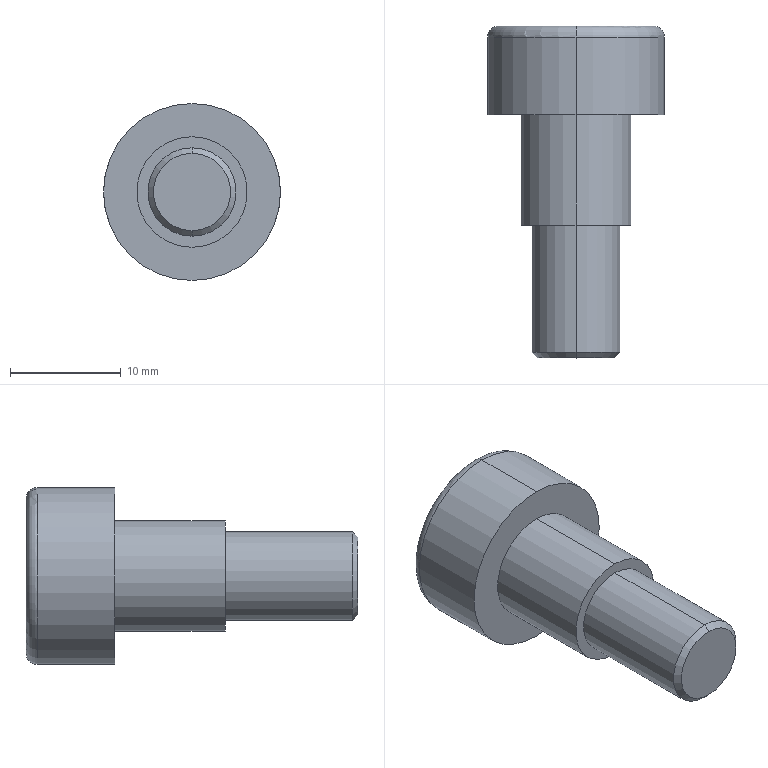Part | STEP file | External thread shoulder bolt MSB10-10 | 1 solid | 21 faces | box 16 x 30 x 16 mm | volume 2915 mm3 | plane 11 | cylinder 6 | torus 2 | cone 2 | commonest cylinder face diameters 8 x2 10 x2 16 x2
STEP:
#1=CARTESIAN_POINT('',(0.,0.,0.));
#2=DIRECTION('',(0.,0.,1.));
#3=DIRECTION('',(1.,0.,0.));
#4=AXIS2_PLACEMENT_3D('',#1,#2,#3);
#5=CARTESIAN_POINT('',(0.,29.,-8.));
#6=VERTEX_POINT('',#5);
#7=CARTESIAN_POINT('',(0.,29.,8.));
#8=VERTEX_POINT('',#7);
#9=CARTESIAN_POINT('',(0.,29.,0.));
#10=DIRECTION('',(0.,-1.,0.));
#11=DIRECTION('',(0.,0.,1.));
#12=AXIS2_PLACEMENT_3D('',#9,#10,#11);
#13=CIRCLE('',#12,8.);
#14=CARTESIAN_POINT('',(0.,29.,0.));
#15=DIRECTION('',(0.,1.,0.));
#16=DIRECTION('',(0.,0.,1.));
#17=AXIS2_PLACEMENT_3D('',#14,#15,#16);
#18=TOROIDAL_SURFACE('',#17,7.,1.);
#19=CARTESIAN_POINT('',(6.283,0.));
#20=DIRECTION('',(-1.,0.));
#21=VECTOR('',#20,1.);
#22=LINE('',#19,#21);
#23=(GEOMETRIC_REPRESENTATION_CONTEXT(2)PARAMETRIC_REPRESENTATION_CONTEXT()REPRESENTATION_CONTEXT('',''));
#24=DEFINITIONAL_REPRESENTATION('',(#22),#23);
#25=PCURVE('',#18,#24);
#26=CARTESIAN_POINT('',(0.,0.,0.));
#27=DIRECTION('',(0.,-1.,0.));
#28=DIRECTION('',(0.,0.,-1.));
#29=AXIS2_PLACEMENT_3D('',#26,#27,#28);
#30=CYLINDRICAL_SURFACE('',#29,8.);
#31=CARTESIAN_POINT('',(-3.142,-29.));
#32=DIRECTION('',(1.,0.));
#33=VECTOR('',#32,1.);
#34=LINE('',#31,#33);
#35=(GEOMETRIC_REPRESENTATION_CONTEXT(2)PARAMETRIC_REPRESENTATION_CONTEXT()REPRESENTATION_CONTEXT('',''));
#36=DEFINITIONAL_REPRESENTATION('',(#34),#35);
#37=PCURVE('',#30,#36);
#38=SURFACE_CURVE('',#13,(#25,#37),.PCURVE_S1.);
#39=EDGE_CURVE('',#6,#8,#38,.T.);
#40=ORIENTED_EDGE('',*,*,#39,.F.);
#41=CARTESIAN_POINT('',(0.,30.,-7.));
#42=VERTEX_POINT('',#41);
#43=CARTESIAN_POINT('',(0.,29.,-7.));
#44=DIRECTION('',(1.,0.,0.));
#45=DIRECTION('',(0.,0.,-1.));
#46=AXIS2_PLACEMENT_3D('',#43,#44,#45);
#47=CIRCLE('',#46,1.);
#48=CARTESIAN_POINT('',(3.142,0.));
#49=DIRECTION('',(0.,1.));
#50=VECTOR('',#49,1.);
#51=LINE('',#48,#50);
#52=(GEOMETRIC_REPRESENTATION_CONTEXT(2)PARAMETRIC_REPRESENTATION_CONTEXT()REPRESENTATION_CONTEXT('',''));
#53=DEFINITIONAL_REPRESENTATION('',(#51),#52);
#54=PCURVE('',#18,#53);
#55=CARTESIAN_POINT('',(0.,29.,0.));
#56=DIRECTION('',(0.,1.,0.));
#57=DIRECTION('',(0.,0.,1.));
#58=AXIS2_PLACEMENT_3D('',#55,#56,#57);
#59=TOROIDAL_SURFACE('',#58,7.,1.);
#60=CARTESIAN_POINT('',(3.142,0.));
#61=DIRECTION('',(0.,1.));
#62=VECTOR('',#61,1.);
#63=LINE('',#60,#62);
#64=(GEOMETRIC_REPRESENTATION_CONTEXT(2)PARAMETRIC_REPRESENTATION_CONTEXT()REPRESENTATION_CONTEXT('',''));
#65=DEFINITIONAL_REPRESENTATION('',(#63),#64);
#66=PCURVE('',#59,#65);
#67=SURFACE_CURVE('',#47,(#54,#66),.PCURVE_S1.);
#68=EDGE_CURVE('',#6,#42,#67,.T.);
#69=ORIENTED_EDGE('',*,*,#68,.T.);
#70=CARTESIAN_POINT('',(0.,30.,7.));
#71=VERTEX_POINT('',#70);
#72=CARTESIAN_POINT('',(0.,30.,0.));
#73=DIRECTION('',(0.,1.,0.));
#74=DIRECTION('',(0.,0.,1.));
#75=AXIS2_PLACEMENT_3D('',#72,#73,#74);
#76=CIRCLE('',#75,7.);
#77=CARTESIAN_POINT('',(0.,1.571));
#78=DIRECTION('',(1.,0.));
#79=VECTOR('',#78,1.);
#80=LINE('',#77,#79);
#81=(GEOMETRIC_REPRESENTATION_CONTEXT(2)PARAMETRIC_REPRESENTATION_CONTEXT()REPRESENTATION_CONTEXT('',''));
#82=DEFINITIONAL_REPRESENTATION('',(#80),#81);
#83=PCURVE('',#18,#82);
#84=CARTESIAN_POINT('',(0.,30.,0.));
#85=DIRECTION('',(0.,1.,0.));
#86=DIRECTION('',(0.,0.,1.));
#87=AXIS2_PLACEMENT_3D('',#84,#85,#86);
#88=PLANE('',#87);
#89=CARTESIAN_POINT('',(0.,0.));
#90=DIRECTION('',(1.,0.));
#91=AXIS2_PLACEMENT_2D('',#89,#90);
#92=CIRCLE('',#91,7.);
#93=(GEOMETRIC_REPRESENTATION_CONTEXT(2)PARAMETRIC_REPRESENTATION_CONTEXT()REPRESENTATION_CONTEXT('',''));
#94=DEFINITIONAL_REPRESENTATION('',(#92),#93);
#95=PCURVE('',#88,#94);
#96=SURFACE_CURVE('',#76,(#83,#95),.PCURVE_S1.);
#97=EDGE_CURVE('',#71,#42,#96,.T.);
#98=ORIENTED_EDGE('',*,*,#97,.F.);
#99=CARTESIAN_POINT('',(0.,29.,7.));
#100=DIRECTION('',(-1.,0.,0.));
#101=DIRECTION('',(0.,0.,1.));
#102=AXIS2_PLACEMENT_3D('',#99,#100,#101);
#103=CIRCLE('',#102,1.);
#104=CARTESIAN_POINT('',(0.,0.));
#105=DIRECTION('',(0.,1.));
#106=VECTOR('',#105,1.);
#107=LINE('',#104,#106);
#108=(GEOMETRIC_REPRESENTATION_CONTEXT(2)PARAMETRIC_REPRESENTATION_CONTEXT()REPRESENTATION_CONTEXT('',''));
#109=DEFINITIONAL_REPRESENTATION('',(#107),#108);
#110=PCURVE('',#18,#109);
#111=CARTESIAN_POINT('',(6.283,0.));
#112=DIRECTION('',(0.,1.));
#113=VECTOR('',#112,1.);
#114=LINE('',#111,#113);
#115=(GEOMETRIC_REPRESENTATION_CONTEXT(2)PARAMETRIC_REPRESENTATION_CONTEXT()REPRESENTATION_CONTEXT('',''));
#116=DEFINITIONAL_REPRESENTATION('',(#114),#115);
#117=PCURVE('',#59,#116);
#118=SURFACE_CURVE('',#103,(#110,#117),.PCURVE_S1.);
#119=EDGE_CURVE('',#8,#71,#118,.T.);
#120=ORIENTED_EDGE('',*,*,#119,.F.);
#121=EDGE_LOOP('',(#40,#69,#98,#120));
#122=FACE_BOUND('',#121,.T.);
#123=ADVANCED_FACE('',(#122),#18,.T.);
#124=CARTESIAN_POINT('',(0.,0.,-3.5));
#125=VERTEX_POINT('',#124);
#126=CARTESIAN_POINT('',(0.,0.,3.5));
#127=VERTEX_POINT('',#126);
#128=CARTESIAN_POINT('',(0.,0.,0.));
#129=DIRECTION('',(0.,-1.,0.));
#130=DIRECTION('',(0.,0.,-1.));
#131=AXIS2_PLACEMENT_3D('',#128,#129,#130);
#132=CIRCLE('',#131,3.5);
#133=CARTESIAN_POINT('',(0.,0.,0.));
#134=DIRECTION('',(0.,1.,0.));
#135=DIRECTION('',(0.,0.,1.));
#136=AXIS2_PLACEMENT_3D('',#133,#134,#135);
#137=CONICAL_SURFACE('',#136,3.5,0.7854);
#138=CARTESIAN_POINT('',(3.142,0.));
#139=DIRECTION('',(-1.,0.));
#140=VECTOR('',#139,1.);
#141=LINE('',#138,#140);
#142=(GEOMETRIC_REPRESENTATION_CONTEXT(2)PARAMETRIC_REPRESENTATION_CONTEXT()REPRESENTATION_CONTEXT('',''));
#143=DEFINITIONAL_REPRESENTATION('',(#141),#142);
#144=PCURVE('',#137,#143);
#145=CARTESIAN_POINT('',(4.,0.,0.));
#146=DIRECTION('',(0.,-1.,0.));
#147=DIRECTION('',(0.,0.,-1.));
#148=AXIS2_PLACEMENT_3D('',#145,#146,#147);
#149=PLANE('',#148);
#150=CARTESIAN_POINT('',(0.,-4.));
#151=DIRECTION('',(1.,0.));
#152=AXIS2_PLACEMENT_2D('',#150,#151);
#153=CIRCLE('',#152,3.5);
#154=(GEOMETRIC_REPRESENTATION_CONTEXT(2)PARAMETRIC_REPRESENTATION_CONTEXT()REPRESENTATION_CONTEXT('',''));
#155=DEFINITIONAL_REPRESENTATION('',(#153),#154);
#156=PCURVE('',#149,#155);
#157=SURFACE_CURVE('',#132,(#144,#156),.PCURVE_S1.);
#158=EDGE_CURVE('',#125,#127,#157,.T.);
#159=ORIENTED_EDGE('',*,*,#158,.F.);
#160=CARTESIAN_POINT('',(0.,0.5,-4.));
#161=VERTEX_POINT('',#160);
#162=CARTESIAN_POINT('',(0.,0.,-3.5));
#163=DIRECTION('',(0.,0.7071,-0.7071));
#164=VECTOR('',#163,1.);
#165=LINE('',#162,#164);
#166=CARTESIAN_POINT('',(3.142,0.));
#167=DIRECTION('',(0.,1.));
#168=VECTOR('',#167,1.);
#169=LINE('',#166,#168);
#170=(GEOMETRIC_REPRESENTATION_CONTEXT(2)PARAMETRIC_REPRESENTATION_CONTEXT()REPRESENTATION_CONTEXT('',''));
#171=DEFINITIONAL_REPRESENTATION('',(#169),#170);
#172=PCURVE('',#137,#171);
#173=CARTESIAN_POINT('',(0.,0.,0.));
#174=DIRECTION('',(0.,1.,0.));
#175=DIRECTION('',(0.,0.,1.));
#176=AXIS2_PLACEMENT_3D('',#173,#174,#175);
#177=CONICAL_SURFACE('',#176,3.5,0.7854);
#178=CARTESIAN_POINT('',(3.142,0.));
#179=DIRECTION('',(0.,1.));
#180=VECTOR('',#179,1.);
#181=LINE('',#178,#180);
#182=(GEOMETRIC_REPRESENTATION_CONTEXT(2)PARAMETRIC_REPRESENTATION_CONTEXT()REPRESENTATION_CONTEXT('',''));
#183=DEFINITIONAL_REPRESENTATION('',(#181),#182);
#184=PCURVE('',#177,#183);
#185=SURFACE_CURVE('',#165,(#172,#184),.PCURVE_S1.);
#186=EDGE_CURVE('',#125,#161,#185,.T.);
#187=ORIENTED_EDGE('',*,*,#186,.T.);
#188=CARTESIAN_POINT('',(0.,0.5,4.));
#189=VERTEX_POINT('',#188);
#190=CARTESIAN_POINT('',(0.,0.5,0.));
#191=DIRECTION('',(0.,1.,0.));
#192=DIRECTION('',(0.,0.,-1.));
#193=AXIS2_PLACEMENT_3D('',#190,#191,#192);
#194=CIRCLE('',#193,4.);
#195=CARTESIAN_POINT('',(-3.142,0.5));
#196=DIRECTION('',(1.,0.));
#197=VECTOR('',#196,1.);
#198=LINE('',#195,#197);
#199=(GEOMETRIC_REPRESENTATION_CONTEXT(2)PARAMETRIC_REPRESENTATION_CONTEXT()REPRESENTATION_CONTEXT('',''));
#200=DEFINITIONAL_REPRESENTATION('',(#198),#199);
#201=PCURVE('',#137,#200);
#202=CARTESIAN_POINT('',(0.,0.,0.));
#203=DIRECTION('',(0.,-1.,0.));
#204=DIRECTION('',(0.,0.,-1.));
#205=AXIS2_PLACEMENT_3D('',#202,#203,#204);
#206=CYLINDRICAL_SURFACE('',#205,4.);
#207=CARTESIAN_POINT('',(6.283,-0.5));
#208=DIRECTION('',(-1.,0.));
#209=VECTOR('',#208,1.);
#210=LINE('',#207,#209);
#211=(GEOMETRIC_REPRESENTATION_CONTEXT(2)PARAMETRIC_REPRESENTATION_CONTEXT()REPRESENTATION_CONTEXT('',''));
#212=DEFINITIONAL_REPRESENTATION('',(#210),#211);
#213=PCURVE('',#206,#212);
#214=SURFACE_CURVE('',#194,(#201,#213),.PCURVE_S1.);
#215=EDGE_CURVE('',#189,#161,#214,.T.);
#216=ORIENTED_EDGE('',*,*,#215,.F.);
#217=CARTESIAN_POINT('',(0.,0.,3.5));
#218=DIRECTION('',(0.,0.7071,0.7071));
#219=VECTOR('',#218,1.);
#220=LINE('',#217,#219);
#221=CARTESIAN_POINT('',(0.,0.));
#222=DIRECTION('',(0.,1.));
#223=VECTOR('',#222,1.);
#224=LINE('',#221,#223);
#225=(GEOMETRIC_REPRESENTATION_CONTEXT(2)PARAMETRIC_REPRESENTATION_CONTEXT()REPRESENTATION_CONTEXT('',''));
#226=DEFINITIONAL_REPRESENTATION('',(#224),#225);
#227=PCURVE('',#137,#226);
#228=CARTESIAN_POINT('',(6.283,0.));
#229=DIRECTION('',(0.,1.));
#230=VECTOR('',#229,1.);
#231=LINE('',#228,#230);
#232=(GEOMETRIC_REPRESENTATION_CONTEXT(2)PARAMETRIC_REPRESENTATION_CONTEXT()REPRESENTATION_CONTEXT('',''));
#233=DEFINITIONAL_REPRESENTATION('',(#231),#232);
#234=PCURVE('',#177,#233);
#235=SURFACE_CURVE('',#220,(#227,#234),.PCURVE_S1.);
#236=EDGE_CURVE('',#127,#189,#235,.T.);
#237=ORIENTED_EDGE('',*,*,#236,.F.);
#238=EDGE_LOOP('',(#159,#187,#216,#237));
#239=FACE_BOUND('',#238,.T.);
#240=ADVANCED_FACE('',(#239),#137,.T.);
#241=CARTESIAN_POINT('',(0.,12.,-4.));
#242=VERTEX_POINT('',#241);
#243=CARTESIAN_POINT('',(0.,12.,4.));
#244=VERTEX_POINT('',#243);
#245=CARTESIAN_POINT('',(0.,12.,0.));
#246=DIRECTION('',(0.,-1.,0.));
#247=DIRECTION('',(0.,0.,-1.));
#248=AXIS2_PLACEMENT_3D('',#245,#246,#247);
#249=CIRCLE('',#248,4.);
#250=CARTESIAN_POINT('',(0.,-12.));
#251=DIRECTION('',(1.,0.));
#252=VECTOR('',#251,1.);
#253=LINE('',#250,#252);
#254=(GEOMETRIC_REPRESENTATION_CONTEXT(2)PARAMETRIC_REPRESENTATION_CONTEXT()REPRESENTATION_CONTEXT('',''));
#255=DEFINITIONAL_REPRESENTATION('',(#253),#254);
#256=PCURVE('',#206,#255);
#257=CARTESIAN_POINT('',(5.,12.,0.));
#258=DIRECTION('',(0.,-1.,0.));
#259=DIRECTION('',(0.,0.,-1.));
#260=AXIS2_PLACEMENT_3D('',#257,#258,#259);
#261=PLANE('',#260);
#262=CARTESIAN_POINT('',(0.,-5.));
#263=DIRECTION('',(1.,0.));
#264=AXIS2_PLACEMENT_2D('',#262,#263);
#265=CIRCLE('',#264,4.);
#266=(GEOMETRIC_REPRESENTATION_CONTEXT(2)PARAMETRIC_REPRESENTATION_CONTEXT()REPRESENTATION_CONTEXT('',''));
#267=DEFINITIONAL_REPRESENTATION('',(#265),#266);
#268=PCURVE('',#261,#267);
#269=SURFACE_CURVE('',#249,(#256,#268),.PCURVE_S1.);
#270=EDGE_CURVE('',#242,#244,#269,.T.);
#271=ORIENTED_EDGE('',*,*,#270,.T.);
#272=CARTESIAN_POINT('',(0.,0.,4.));
#273=DIRECTION('',(0.,-1.,0.));
#274=VECTOR('',#273,1.);
#275=LINE('',#272,#274);
#276=CARTESIAN_POINT('',(3.142,0.));
#277=DIRECTION('',(0.,1.));
#278=VECTOR('',#277,1.);
#279=LINE('',#276,#278);
#280=(GEOMETRIC_REPRESENTATION_CONTEXT(2)PARAMETRIC_REPRESENTATION_CONTEXT()REPRESENTATION_CONTEXT('',''));
#281=DEFINITIONAL_REPRESENTATION('',(#279),#280);
#282=PCURVE('',#206,#281);
#283=CARTESIAN_POINT('',(0.,0.,0.));
#284=DIRECTION('',(0.,-1.,0.));
#285=DIRECTION('',(0.,0.,-1.));
#286=AXIS2_PLACEMENT_3D('',#283,#284,#285);
#287=CYLINDRICAL_SURFACE('',#286,4.);
#288=CARTESIAN_POINT('',(3.142,0.));
#289=DIRECTION('',(0.,1.));
#290=VECTOR('',#289,1.);
#291=LINE('',#288,#290);
#292=(GEOMETRIC_REPRESENTATION_CONTEXT(2)PARAMETRIC_REPRESENTATION_CONTEXT()REPRESENTATION_CONTEXT('',''));
#293=DEFINITIONAL_REPRESENTATION('',(#291),#292);
#294=PCURVE('',#287,#293);
#295=SURFACE_CURVE('',#275,(#282,#294),.PCURVE_S1.);
#296=EDGE_CURVE('',#244,#189,#295,.T.);
#297=ORIENTED_EDGE('',*,*,#296,.T.);
#298=ORIENTED_EDGE('',*,*,#215,.T.);
#299=CARTESIAN_POINT('',(0.,0.,-4.));
#300=DIRECTION('',(0.,-1.,0.));
#301=VECTOR('',#300,1.);
#302=LINE('',#299,#301);
#303=CARTESIAN_POINT('',(0.,0.));
#304=DIRECTION('',(0.,1.));
#305=VECTOR('',#304,1.);
#306=LINE('',#303,#305);
#307=(GEOMETRIC_REPRESENTATION_CONTEXT(2)PARAMETRIC_REPRESENTATION_CONTEXT()REPRESENTATION_CONTEXT('',''));
#308=DEFINITIONAL_REPRESENTATION('',(#306),#307);
#309=PCURVE('',#206,#308);
#310=CARTESIAN_POINT('',(6.283,0.));
#311=DIRECTION('',(0.,1.));
#312=VECTOR('',#311,1.);
#313=LINE('',#310,#312);
#314=(GEOMETRIC_REPRESENTATION_CONTEXT(2)PARAMETRIC_REPRESENTATION_CONTEXT()REPRESENTATION_CONTEXT('',''));
#315=DEFINITIONAL_REPRESENTATION('',(#313),#314);
#316=PCURVE('',#287,#315);
#317=SURFACE_CURVE('',#302,(#309,#316),.PCURVE_S1.);
#318=EDGE_CURVE('',#242,#161,#317,.T.);
#319=ORIENTED_EDGE('',*,*,#318,.F.);
#320=EDGE_LOOP('',(#271,#297,#298,#319));
#321=FACE_BOUND('',#320,.T.);
#322=ADVANCED_FACE('',(#321),#206,.T.);
#323=CARTESIAN_POINT('',(0.,22.,-5.));
#324=VERTEX_POINT('',#323);
#325=CARTESIAN_POINT('',(0.,22.,5.));
#326=VERTEX_POINT('',#325);
#327=CARTESIAN_POINT('',(0.,22.,0.));
#328=DIRECTION('',(0.,-1.,0.));
#329=DIRECTION('',(0.,0.,-1.));
#330=AXIS2_PLACEMENT_3D('',#327,#328,#329);
#331=CIRCLE('',#330,5.);
#332=CARTESIAN_POINT('',(0.,0.,0.));
#333=DIRECTION('',(0.,-1.,0.));
#334=DIRECTION('',(0.,0.,-1.));
#335=AXIS2_PLACEMENT_3D('',#332,#333,#334);
#336=CYLINDRICAL_SURFACE('',#335,5.);
#337=CARTESIAN_POINT('',(0.,-22.));
#338=DIRECTION('',(1.,0.));
#339=VECTOR('',#338,1.);
#340=LINE('',#337,#339);
#341=(GEOMETRIC_REPRESENTATION_CONTEXT(2)PARAMETRIC_REPRESENTATION_CONTEXT()REPRESENTATION_CONTEXT('',''));
#342=DEFINITIONAL_REPRESENTATION('',(#340),#341);
#343=PCURVE('',#336,#342);
#344=CARTESIAN_POINT('',(8.,22.,0.));
#345=DIRECTION('',(0.,-1.,0.));
#346=DIRECTION('',(0.,0.,-1.));
#347=AXIS2_PLACEMENT_3D('',#344,#345,#346);
#348=PLANE('',#347);
#349=CARTESIAN_POINT('',(0.,-8.));
#350=DIRECTION('',(1.,0.));
#351=AXIS2_PLACEMENT_2D('',#349,#350);
#352=CIRCLE('',#351,5.);
#353=(GEOMETRIC_REPRESENTATION_CONTEXT(2)PARAMETRIC_REPRESENTATION_CONTEXT()REPRESENTATION_CONTEXT('',''));
#354=DEFINITIONAL_REPRESENTATION('',(#352),#353);
#355=PCURVE('',#348,#354);
#356=SURFACE_CURVE('',#331,(#343,#355),.PCURVE_S1.);
#357=EDGE_CURVE('',#324,#326,#356,.T.);
#358=ORIENTED_EDGE('',*,*,#357,.T.);
#359=CARTESIAN_POINT('',(0.,12.,5.));
#360=VERTEX_POINT('',#359);
#361=CARTESIAN_POINT('',(0.,0.,5.));
#362=DIRECTION('',(0.,-1.,0.));
#363=VECTOR('',#362,1.);
#364=LINE('',#361,#363);
#365=CARTESIAN_POINT('',(3.142,0.));
#366=DIRECTION('',(0.,1.));
#367=VECTOR('',#366,1.);
#368=LINE('',#365,#367);
#369=(GEOMETRIC_REPRESENTATION_CONTEXT(2)PARAMETRIC_REPRESENTATION_CONTEXT()REPRESENTATION_CONTEXT('',''));
#370=DEFINITIONAL_REPRESENTATION('',(#368),#369);
#371=PCURVE('',#336,#370);
#372=CARTESIAN_POINT('',(0.,0.,0.));
#373=DIRECTION('',(0.,-1.,0.));
#374=DIRECTION('',(0.,0.,-1.));
#375=AXIS2_PLACEMENT_3D('',#372,#373,#374);
#376=CYLINDRICAL_SURFACE('',#375,5.);
#377=CARTESIAN_POINT('',(3.142,0.));
#378=DIRECTION('',(0.,1.));
#379=VECTOR('',#378,1.);
#380=LINE('',#377,#379);
#381=(GEOMETRIC_REPRESENTATION_CONTEXT(2)PARAMETRIC_REPRESENTATION_CONTEXT()REPRESENTATION_CONTEXT('',''));
#382=DEFINITIONAL_REPRESENTATION('',(#380),#381);
#383=PCURVE('',#376,#382);
#384=SURFACE_CURVE('',#364,(#371,#383),.PCURVE_S1.);
#385=EDGE_CURVE('',#326,#360,#384,.T.);
#386=ORIENTED_EDGE('',*,*,#385,.T.);
#387=CARTESIAN_POINT('',(0.,12.,-5.));
#388=VERTEX_POINT('',#387);
#389=CARTESIAN_POINT('',(0.,12.,0.));
#390=DIRECTION('',(0.,-1.,0.));
#391=DIRECTION('',(0.,0.,-1.));
#392=AXIS2_PLACEMENT_3D('',#389,#390,#391);
#393=CIRCLE('',#392,5.);
#394=CARTESIAN_POINT('',(0.,-12.));
#395=DIRECTION('',(1.,0.));
#396=VECTOR('',#395,1.);
#397=LINE('',#394,#396);
#398=(GEOMETRIC_REPRESENTATION_CONTEXT(2)PARAMETRIC_REPRESENTATION_CONTEXT()REPRESENTATION_CONTEXT('',''));
#399=DEFINITIONAL_REPRESENTATION('',(#397),#398);
#400=PCURVE('',#336,#399);
#401=CARTESIAN_POINT('',(0.,-5.));
#402=DIRECTION('',(1.,0.));
#403=AXIS2_PLACEMENT_2D('',#401,#402);
#404=CIRCLE('',#403,5.);
#405=(GEOMETRIC_REPRESENTATION_CONTEXT(2)PARAMETRIC_REPRESENTATION_CONTEXT()REPRESENTATION_CONTEXT('',''));
#406=DEFINITIONAL_REPRESENTATION('',(#404),#405);
#407=PCURVE('',#261,#406);
#408=SURFACE_CURVE('',#393,(#400,#407),.PCURVE_S1.);
#409=EDGE_CURVE('',#388,#360,#408,.T.);
#410=ORIENTED_EDGE('',*,*,#409,.F.);
#411=CARTESIAN_POINT('',(0.,0.,-5.));
#412=DIRECTION('',(0.,-1.,0.));
#413=VECTOR('',#412,1.);
#414=LINE('',#411,#413);
#415=CARTESIAN_POINT('',(0.,0.));
#416=DIRECTION('',(0.,1.));
#417=VECTOR('',#416,1.);
#418=LINE('',#415,#417);
#419=(GEOMETRIC_REPRESENTATION_CONTEXT(2)PARAMETRIC_REPRESENTATION_CONTEXT()REPRESENTATION_CONTEXT('',''));
#420=DEFINITIONAL_REPRESENTATION('',(#418),#419);
#421=PCURVE('',#336,#420);
#422=CARTESIAN_POINT('',(6.283,0.));
#423=DIRECTION('',(0.,1.));
#424=VECTOR('',#423,1.);
#425=LINE('',#422,#424);
#426=(GEOMETRIC_REPRESENTATION_CONTEXT(2)PARAMETRIC_REPRESENTATION_CONTEXT()REPRESENTATION_CONTEXT('',''));
#427=DEFINITIONAL_REPRESENTATION('',(#425),#426);
#428=PCURVE('',#376,#427);
#429=SURFACE_CURVE('',#414,(#421,#428),.PCURVE_S1.);
#430=EDGE_CURVE('',#324,#388,#429,.T.);
#431=ORIENTED_EDGE('',*,*,#430,.F.);
#432=EDGE_LOOP('',(#358,#386,#410,#431));
#433=FACE_BOUND('',#432,.T.);
#434=ADVANCED_FACE('',(#433),#336,.T.);
#435=ORIENTED_EDGE('',*,*,#39,.T.);
#436=CARTESIAN_POINT('',(0.,22.,8.));
#437=VERTEX_POINT('',#436);
#438=CARTESIAN_POINT('',(0.,0.,8.));
#439=DIRECTION('',(0.,-1.,0.));
#440=VECTOR('',#439,1.);
#441=LINE('',#438,#440);
#442=CARTESIAN_POINT('',(3.142,0.));
#443=DIRECTION('',(0.,1.));
#444=VECTOR('',#443,1.);
#445=LINE('',#442,#444);
#446=(GEOMETRIC_REPRESENTATION_CONTEXT(2)PARAMETRIC_REPRESENTATION_CONTEXT()REPRESENTATION_CONTEXT('',''));
#447=DEFINITIONAL_REPRESENTATION('',(#445),#446);
#448=PCURVE('',#30,#447);
#449=CARTESIAN_POINT('',(0.,0.,0.));
#450=DIRECTION('',(0.,-1.,0.));
#451=DIRECTION('',(0.,0.,-1.));
#452=AXIS2_PLACEMENT_3D('',#449,#450,#451);
#453=CYLINDRICAL_SURFACE('',#452,8.);
#454=CARTESIAN_POINT('',(3.142,0.));
#455=DIRECTION('',(0.,1.));
#456=VECTOR('',#455,1.);
#457=LINE('',#454,#456);
#458=(GEOMETRIC_REPRESENTATION_CONTEXT(2)PARAMETRIC_REPRESENTATION_CONTEXT()REPRESENTATION_CONTEXT('',''));
#459=DEFINITIONAL_REPRESENTATION('',(#457),#458);
#460=PCURVE('',#453,#459);
#461=SURFACE_CURVE('',#441,(#448,#460),.PCURVE_S1.);
#462=EDGE_CURVE('',#8,#437,#461,.T.);
#463=ORIENTED_EDGE('',*,*,#462,.T.);
#464=CARTESIAN_POINT('',(0.,22.,-8.));
#465=VERTEX_POINT('',#464);
#466=CARTESIAN_POINT('',(0.,22.,0.));
#467=DIRECTION('',(0.,-1.,0.));
#468=DIRECTION('',(0.,0.,-1.));
#469=AXIS2_PLACEMENT_3D('',#466,#467,#468);
#470=CIRCLE('',#469,8.);
#471=CARTESIAN_POINT('',(0.,-22.));
#472=DIRECTION('',(1.,0.));
#473=VECTOR('',#472,1.);
#474=LINE('',#471,#473);
#475=(GEOMETRIC_REPRESENTATION_CONTEXT(2)PARAMETRIC_REPRESENTATION_CONTEXT()REPRESENTATION_CONTEXT('',''));
#476=DEFINITIONAL_REPRESENTATION('',(#474),#475);
#477=PCURVE('',#30,#476);
#478=CARTESIAN_POINT('',(0.,-8.));
#479=DIRECTION('',(1.,0.));
#480=AXIS2_PLACEMENT_2D('',#478,#479);
#481=CIRCLE('',#480,8.);
#482=(GEOMETRIC_REPRESENTATION_CONTEXT(2)PARAMETRIC_REPRESENTATION_CONTEXT()REPRESENTATION_CONTEXT('',''));
#483=DEFINITIONAL_REPRESENTATION('',(#481),#482);
#484=PCURVE('',#348,#483);
#485=SURFACE_CURVE('',#470,(#477,#484),.PCURVE_S1.);
#486=EDGE_CURVE('',#465,#437,#485,.T.);
#487=ORIENTED_EDGE('',*,*,#486,.F.);
#488=CARTESIAN_POINT('',(0.,0.,-8.));
#489=DIRECTION('',(0.,-1.,0.));
#490=VECTOR('',#489,1.);
#491=LINE('',#488,#490);
#492=CARTESIAN_POINT('',(0.,0.));
#493=DIRECTION('',(0.,1.));
#494=VECTOR('',#493,1.);
#495=LINE('',#492,#494);
#496=(GEOMETRIC_REPRESENTATION_CONTEXT(2)PARAMETRIC_REPRESENTATION_CONTEXT()REPRESENTATION_CONTEXT('',''));
#497=DEFINITIONAL_REPRESENTATION('',(#495),#496);
#498=PCURVE('',#30,#497);
#499=CARTESIAN_POINT('',(6.283,0.));
#500=DIRECTION('',(0.,1.));
#501=VECTOR('',#500,1.);
#502=LINE('',#499,#501);
#503=(GEOMETRIC_REPRESENTATION_CONTEXT(2)PARAMETRIC_REPRESENTATION_CONTEXT()REPRESENTATION_CONTEXT('',''));
#504=DEFINITIONAL_REPRESENTATION('',(#502),#503);
#505=PCURVE('',#453,#504);
#506=SURFACE_CURVE('',#491,(#498,#505),.PCURVE_S1.);
#507=EDGE_CURVE('',#6,#465,#506,.T.);
#508=ORIENTED_EDGE('',*,*,#507,.F.);
#509=EDGE_LOOP('',(#435,#463,#487,#508));
#510=FACE_BOUND('',#509,.T.);
#511=ADVANCED_FACE('',(#510),#30,.T.);
#512=CARTESIAN_POINT('',(0.,0.,0.));
#513=DIRECTION('',(0.,-1.,0.));
#514=DIRECTION('',(0.,0.,-1.));
#515=AXIS2_PLACEMENT_3D('',#512,#513,#514);
#516=CIRCLE('',#515,3.5);
#517=CARTESIAN_POINT('',(0.,-4.));
#518=DIRECTION('',(1.,0.));
#519=AXIS2_PLACEMENT_2D('',#517,#518);
#520=CIRCLE('',#519,3.5);
#521=(GEOMETRIC_REPRESENTATION_CONTEXT(2)PARAMETRIC_REPRESENTATION_CONTEXT()REPRESENTATION_CONTEXT('',''));
#522=DEFINITIONAL_REPRESENTATION('',(#520),#521);
#523=PCURVE('',#149,#522);
#524=CARTESIAN_POINT('',(9.425,0.));
#525=DIRECTION('',(-1.,0.));
#526=VECTOR('',#525,1.);
#527=LINE('',#524,#526);
#528=(GEOMETRIC_REPRESENTATION_CONTEXT(2)PARAMETRIC_REPRESENTATION_CONTEXT()REPRESENTATION_CONTEXT('',''));
#529=DEFINITIONAL_REPRESENTATION('',(#527),#528);
#530=PCURVE('',#177,#529);
#531=SURFACE_CURVE('',#516,(#523,#530),.PCURVE_S1.);
#532=EDGE_CURVE('',#127,#125,#531,.T.);
#533=ORIENTED_EDGE('',*,*,#532,.T.);
#534=ORIENTED_EDGE('',*,*,#158,.T.);
#535=EDGE_LOOP('',(#533,#534));
#536=FACE_BOUND('',#535,.T.);
#537=ADVANCED_FACE('',(#536),#149,.T.);
#538=CARTESIAN_POINT('',(1.732,30.,3.));
#539=VERTEX_POINT('',#538);
#540=CARTESIAN_POINT('',(3.464,30.,0.));
#541=VERTEX_POINT('',#540);
#542=CARTESIAN_POINT('',(1.732,30.,3.));
#543=DIRECTION('',(0.5,0.,-0.866));
#544=VECTOR('',#543,1.);
#545=LINE('',#542,#544);
#546=CARTESIAN_POINT('',(3.,1.732));
#547=DIRECTION('',(-0.866,0.5));
#548=VECTOR('',#547,1.);
#549=LINE('',#546,#548);
#550=(GEOMETRIC_REPRESENTATION_CONTEXT(2)PARAMETRIC_REPRESENTATION_CONTEXT()REPRESENTATION_CONTEXT('',''));
#551=DEFINITIONAL_REPRESENTATION('',(#549),#550);
#552=PCURVE('',#88,#551);
#553=CARTESIAN_POINT('',(1.732,27.8,3.));
#554=DIRECTION('',(0.866,0.,0.5));
#555=DIRECTION('',(0.5,0.,-0.866));
#556=AXIS2_PLACEMENT_3D('',#553,#554,#555);
#557=PLANE('',#556);
#558=CARTESIAN_POINT('',(0.,2.2));
#559=DIRECTION('',(1.,0.));
#560=VECTOR('',#559,1.);
#561=LINE('',#558,#560);
#562=(GEOMETRIC_REPRESENTATION_CONTEXT(2)PARAMETRIC_REPRESENTATION_CONTEXT()REPRESENTATION_CONTEXT('',''));
#563=DEFINITIONAL_REPRESENTATION('',(#561),#562);
#564=PCURVE('',#557,#563);
#565=SURFACE_CURVE('',#545,(#552,#564),.PCURVE_S1.);
#566=EDGE_CURVE('',#539,#541,#565,.T.);
#567=ORIENTED_EDGE('',*,*,#566,.F.);
#568=CARTESIAN_POINT('',(-1.732,30.,3.));
#569=VERTEX_POINT('',#568);
#570=CARTESIAN_POINT('',(-1.732,30.,3.));
#571=DIRECTION('',(1.,0.,0.));
#572=VECTOR('',#571,1.);
#573=LINE('',#570,#572);
#574=CARTESIAN_POINT('',(3.,-1.732));
#575=DIRECTION('',(0.,1.));
#576=VECTOR('',#575,1.);
#577=LINE('',#574,#576);
#578=(GEOMETRIC_REPRESENTATION_CONTEXT(2)PARAMETRIC_REPRESENTATION_CONTEXT()REPRESENTATION_CONTEXT('',''));
#579=DEFINITIONAL_REPRESENTATION('',(#577),#578);
#580=PCURVE('',#88,#579);
#581=CARTESIAN_POINT('',(-1.732,27.8,3.));
#582=DIRECTION('',(0.,0.,1.));
#583=DIRECTION('',(1.,0.,0.));
#584=AXIS2_PLACEMENT_3D('',#581,#582,#583);
#585=PLANE('',#584);
#586=CARTESIAN_POINT('',(0.,2.2));
#587=DIRECTION('',(1.,0.));
#588=VECTOR('',#587,1.);
#589=LINE('',#586,#588);
#590=(GEOMETRIC_REPRESENTATION_CONTEXT(2)PARAMETRIC_REPRESENTATION_CONTEXT()REPRESENTATION_CONTEXT('',''));
#591=DEFINITIONAL_REPRESENTATION('',(#589),#590);
#592=PCURVE('',#585,#591);
#593=SURFACE_CURVE('',#573,(#580,#592),.PCURVE_S1.);
#594=EDGE_CURVE('',#569,#539,#593,.T.);
#595=ORIENTED_EDGE('',*,*,#594,.F.);
#596=CARTESIAN_POINT('',(-3.464,30.,0.));
#597=VERTEX_POINT('',#596);
#598=CARTESIAN_POINT('',(-3.464,30.,0.));
#599=DIRECTION('',(0.5,0.,0.866));
#600=VECTOR('',#599,1.);
#601=LINE('',#598,#600);
#602=CARTESIAN_POINT('',(0.,-3.464));
#603=DIRECTION('',(0.866,0.5));
#604=VECTOR('',#603,1.);
#605=LINE('',#602,#604);
#606=(GEOMETRIC_REPRESENTATION_CONTEXT(2)PARAMETRIC_REPRESENTATION_CONTEXT()REPRESENTATION_CONTEXT('',''));
#607=DEFINITIONAL_REPRESENTATION('',(#605),#606);
#608=PCURVE('',#88,#607);
#609=CARTESIAN_POINT('',(-3.464,27.8,0.));
#610=DIRECTION('',(-0.866,0.,0.5));
#611=DIRECTION('',(0.5,0.,0.866));
#612=AXIS2_PLACEMENT_3D('',#609,#610,#611);
#613=PLANE('',#612);
#614=CARTESIAN_POINT('',(0.,2.2));
#615=DIRECTION('',(1.,0.));
#616=VECTOR('',#615,1.);
#617=LINE('',#614,#616);
#618=(GEOMETRIC_REPRESENTATION_CONTEXT(2)PARAMETRIC_REPRESENTATION_CONTEXT()REPRESENTATION_CONTEXT('',''));
#619=DEFINITIONAL_REPRESENTATION('',(#617),#618);
#620=PCURVE('',#613,#619);
#621=SURFACE_CURVE('',#601,(#608,#620),.PCURVE_S1.);
#622=EDGE_CURVE('',#597,#569,#621,.T.);
#623=ORIENTED_EDGE('',*,*,#622,.F.);
#624=CARTESIAN_POINT('',(-1.732,30.,-3.));
#625=VERTEX_POINT('',#624);
#626=CARTESIAN_POINT('',(-1.732,30.,-3.));
#627=DIRECTION('',(-0.5,0.,0.866));
#628=VECTOR('',#627,1.);
#629=LINE('',#626,#628);
#630=CARTESIAN_POINT('',(-3.,-1.732));
#631=DIRECTION('',(0.866,-0.5));
#632=VECTOR('',#631,1.);
#633=LINE('',#630,#632);
#634=(GEOMETRIC_REPRESENTATION_CONTEXT(2)PARAMETRIC_REPRESENTATION_CONTEXT()REPRESENTATION_CONTEXT('',''));
#635=DEFINITIONAL_REPRESENTATION('',(#633),#634);
#636=PCURVE('',#88,#635);
#637=CARTESIAN_POINT('',(-1.732,27.8,-3.));
#638=DIRECTION('',(-0.866,0.,-0.5));
#639=DIRECTION('',(-0.5,0.,0.866));
#640=AXIS2_PLACEMENT_3D('',#637,#638,#639);
#641=PLANE('',#640);
#642=CARTESIAN_POINT('',(0.,2.2));
#643=DIRECTION('',(1.,0.));
#644=VECTOR('',#643,1.);
#645=LINE('',#642,#644);
#646=(GEOMETRIC_REPRESENTATION_CONTEXT(2)PARAMETRIC_REPRESENTATION_CONTEXT()REPRESENTATION_CONTEXT('',''));
#647=DEFINITIONAL_REPRESENTATION('',(#645),#646);
#648=PCURVE('',#641,#647);
#649=SURFACE_CURVE('',#629,(#636,#648),.PCURVE_S1.);
#650=EDGE_CURVE('',#625,#597,#649,.T.);
#651=ORIENTED_EDGE('',*,*,#650,.F.);
#652=CARTESIAN_POINT('',(1.732,30.,-3.));
#653=VERTEX_POINT('',#652);
#654=CARTESIAN_POINT('',(1.732,30.,-3.));
#655=DIRECTION('',(-1.,0.,0.));
#656=VECTOR('',#655,1.);
#657=LINE('',#654,#656);
#658=CARTESIAN_POINT('',(-3.,1.732));
#659=DIRECTION('',(0.,-1.));
#660=VECTOR('',#659,1.);
#661=LINE('',#658,#660);
#662=(GEOMETRIC_REPRESENTATION_CONTEXT(2)PARAMETRIC_REPRESENTATION_CONTEXT()REPRESENTATION_CONTEXT('',''));
#663=DEFINITIONAL_REPRESENTATION('',(#661),#662);
#664=PCURVE('',#88,#663);
#665=CARTESIAN_POINT('',(1.732,27.8,-3.));
#666=DIRECTION('',(0.,0.,-1.));
#667=DIRECTION('',(-1.,0.,0.));
#668=AXIS2_PLACEMENT_3D('',#665,#666,#667);
#669=PLANE('',#668);
#670=CARTESIAN_POINT('',(0.,2.2));
#671=DIRECTION('',(1.,0.));
#672=VECTOR('',#671,1.);
#673=LINE('',#670,#672);
#674=(GEOMETRIC_REPRESENTATION_CONTEXT(2)PARAMETRIC_REPRESENTATION_CONTEXT()REPRESENTATION_CONTEXT('',''));
#675=DEFINITIONAL_REPRESENTATION('',(#673),#674);
#676=PCURVE('',#669,#675);
#677=SURFACE_CURVE('',#657,(#664,#676),.PCURVE_S1.);
#678=EDGE_CURVE('',#653,#625,#677,.T.);
#679=ORIENTED_EDGE('',*,*,#678,.F.);
#680=CARTESIAN_POINT('',(3.464,30.,0.));
#681=DIRECTION('',(-0.5,0.,-0.866));
#682=VECTOR('',#681,1.);
#683=LINE('',#680,#682);
#684=CARTESIAN_POINT('',(0.,3.464));
#685=DIRECTION('',(-0.866,-0.5));
#686=VECTOR('',#685,1.);
#687=LINE('',#684,#686);
#688=(GEOMETRIC_REPRESENTATION_CONTEXT(2)PARAMETRIC_REPRESENTATION_CONTEXT()REPRESENTATION_CONTEXT('',''));
#689=DEFINITIONAL_REPRESENTATION('',(#687),#688);
#690=PCURVE('',#88,#689);
#691=CARTESIAN_POINT('',(3.464,27.8,0.));
#692=DIRECTION('',(0.866,0.,-0.5));
#693=DIRECTION('',(-0.5,0.,-0.866));
#694=AXIS2_PLACEMENT_3D('',#691,#692,#693);
#695=PLANE('',#694);
#696=CARTESIAN_POINT('',(0.,2.2));
#697=DIRECTION('',(1.,0.));
#698=VECTOR('',#697,1.);
#699=LINE('',#696,#698);
#700=(GEOMETRIC_REPRESENTATION_CONTEXT(2)PARAMETRIC_REPRESENTATION_CONTEXT()REPRESENTATION_CONTEXT('',''));
#701=DEFINITIONAL_REPRESENTATION('',(#699),#700);
#702=PCURVE('',#695,#701);
#703=SURFACE_CURVE('',#683,(#690,#702),.PCURVE_S1.);
#704=EDGE_CURVE('',#541,#653,#703,.T.);
#705=ORIENTED_EDGE('',*,*,#704,.F.);
#706=EDGE_LOOP('',(#567,#595,#623,#651,#679,#705));
#707=FACE_BOUND('',#706,.T.);
#708=ORIENTED_EDGE('',*,*,#97,.T.);
#709=CARTESIAN_POINT('',(0.,30.,0.));
#710=DIRECTION('',(0.,1.,0.));
#711=DIRECTION('',(0.,0.,1.));
#712=AXIS2_PLACEMENT_3D('',#709,#710,#711);
#713=CIRCLE('',#712,7.);
#714=CARTESIAN_POINT('',(0.,0.));
#715=DIRECTION('',(1.,0.));
#716=AXIS2_PLACEMENT_2D('',#714,#715);
#717=CIRCLE('',#716,7.);
#718=(GEOMETRIC_REPRESENTATION_CONTEXT(2)PARAMETRIC_REPRESENTATION_CONTEXT()REPRESENTATION_CONTEXT('',''));
#719=DEFINITIONAL_REPRESENTATION('',(#717),#718);
#720=PCURVE('',#88,#719);
#721=CARTESIAN_POINT('',(0.,1.571));
#722=DIRECTION('',(1.,0.));
#723=VECTOR('',#722,1.);
#724=LINE('',#721,#723);
#725=(GEOMETRIC_REPRESENTATION_CONTEXT(2)PARAMETRIC_REPRESENTATION_CONTEXT()REPRESENTATION_CONTEXT('',''));
#726=DEFINITIONAL_REPRESENTATION('',(#724),#725);
#727=PCURVE('',#59,#726);
#728=SURFACE_CURVE('',#713,(#720,#727),.PCURVE_S1.);
#729=EDGE_CURVE('',#42,#71,#728,.T.);
#730=ORIENTED_EDGE('',*,*,#729,.T.);
#731=EDGE_LOOP('',(#708,#730));
#732=FACE_BOUND('',#731,.T.);
#733=ADVANCED_FACE('',(#707,#732),#88,.T.);
#734=ORIENTED_EDGE('',*,*,#462,.F.);
#735=CARTESIAN_POINT('',(0.,29.,0.));
#736=DIRECTION('',(0.,-1.,0.));
#737=DIRECTION('',(0.,0.,1.));
#738=AXIS2_PLACEMENT_3D('',#735,#736,#737);
#739=CIRCLE('',#738,8.);
#740=CARTESIAN_POINT('',(3.142,-29.));
#741=DIRECTION('',(1.,0.));
#742=VECTOR('',#741,1.);
#743=LINE('',#740,#742);
#744=(GEOMETRIC_REPRESENTATION_CONTEXT(2)PARAMETRIC_REPRESENTATION_CONTEXT()REPRESENTATION_CONTEXT('',''));
#745=DEFINITIONAL_REPRESENTATION('',(#743),#744);
#746=PCURVE('',#453,#745);
#747=CARTESIAN_POINT('',(6.283,0.));
#748=DIRECTION('',(-1.,0.));
#749=VECTOR('',#748,1.);
#750=LINE('',#747,#749);
#751=(GEOMETRIC_REPRESENTATION_CONTEXT(2)PARAMETRIC_REPRESENTATION_CONTEXT()REPRESENTATION_CONTEXT('',''));
#752=DEFINITIONAL_REPRESENTATION('',(#750),#751);
#753=PCURVE('',#59,#752);
#754=SURFACE_CURVE('',#739,(#746,#753),.PCURVE_S1.);
#755=EDGE_CURVE('',#8,#6,#754,.T.);
#756=ORIENTED_EDGE('',*,*,#755,.T.);
#757=ORIENTED_EDGE('',*,*,#507,.T.);
#758=CARTESIAN_POINT('',(0.,22.,0.));
#759=DIRECTION('',(0.,-1.,0.));
#760=DIRECTION('',(0.,0.,-1.));
#761=AXIS2_PLACEMENT_3D('',#758,#759,#760);
#762=CIRCLE('',#761,8.);
#763=CARTESIAN_POINT('',(0.,-22.));
#764=DIRECTION('',(1.,0.));
#765=VECTOR('',#764,1.);
#766=LINE('',#763,#765);
#767=(GEOMETRIC_REPRESENTATION_CONTEXT(2)PARAMETRIC_REPRESENTATION_CONTEXT()REPRESENTATION_CONTEXT('',''));
#768=DEFINITIONAL_REPRESENTATION('',(#766),#767);
#769=PCURVE('',#453,#768);
#770=CARTESIAN_POINT('',(0.,-8.));
#771=DIRECTION('',(1.,0.));
#772=AXIS2_PLACEMENT_2D('',#770,#771);
#773=CIRCLE('',#772,8.);
#774=(GEOMETRIC_REPRESENTATION_CONTEXT(2)PARAMETRIC_REPRESENTATION_CONTEXT()REPRESENTATION_CONTEXT('',''));
#775=DEFINITIONAL_REPRESENTATION('',(#773),#774);
#776=PCURVE('',#348,#775);
#777=SURFACE_CURVE('',#762,(#769,#776),.PCURVE_S1.);
#778=EDGE_CURVE('',#437,#465,#777,.T.);
#779=ORIENTED_EDGE('',*,*,#778,.F.);
#780=EDGE_LOOP('',(#734,#756,#757,#779));
#781=FACE_BOUND('',#780,.T.);
#782=ADVANCED_FACE('',(#781),#453,.T.);
#783=ORIENTED_EDGE('',*,*,#486,.T.);
#784=ORIENTED_EDGE('',*,*,#778,.T.);
#785=EDGE_LOOP('',(#783,#784));
#786=FACE_BOUND('',#785,.T.);
#787=ORIENTED_EDGE('',*,*,#357,.F.);
#788=CARTESIAN_POINT('',(0.,22.,0.));
#789=DIRECTION('',(0.,-1.,0.));
#790=DIRECTION('',(0.,0.,-1.));
#791=AXIS2_PLACEMENT_3D('',#788,#789,#790);
#792=CIRCLE('',#791,5.);
#793=CARTESIAN_POINT('',(0.,-8.));
#794=DIRECTION('',(1.,0.));
#795=AXIS2_PLACEMENT_2D('',#793,#794);
#796=CIRCLE('',#795,5.);
#797=(GEOMETRIC_REPRESENTATION_CONTEXT(2)PARAMETRIC_REPRESENTATION_CONTEXT()REPRESENTATION_CONTEXT('',''));
#798=DEFINITIONAL_REPRESENTATION('',(#796),#797);
#799=PCURVE('',#348,#798);
#800=CARTESIAN_POINT('',(0.,-22.));
#801=DIRECTION('',(1.,0.));
#802=VECTOR('',#801,1.);
#803=LINE('',#800,#802);
#804=(GEOMETRIC_REPRESENTATION_CONTEXT(2)PARAMETRIC_REPRESENTATION_CONTEXT()REPRESENTATION_CONTEXT('',''));
#805=DEFINITIONAL_REPRESENTATION('',(#803),#804);
#806=PCURVE('',#376,#805);
#807=SURFACE_CURVE('',#792,(#799,#806),.PCURVE_S1.);
#808=EDGE_CURVE('',#326,#324,#807,.T.);
#809=ORIENTED_EDGE('',*,*,#808,.F.);
#810=EDGE_LOOP('',(#787,#809));
#811=FACE_BOUND('',#810,.T.);
#812=ADVANCED_FACE('',(#786,#811),#348,.T.);
#813=ORIENTED_EDGE('',*,*,#385,.F.);
#814=ORIENTED_EDGE('',*,*,#808,.T.);
#815=ORIENTED_EDGE('',*,*,#430,.T.);
#816=CARTESIAN_POINT('',(0.,12.,0.));
#817=DIRECTION('',(0.,-1.,0.));
#818=DIRECTION('',(0.,0.,-1.));
#819=AXIS2_PLACEMENT_3D('',#816,#817,#818);
#820=CIRCLE('',#819,5.);
#821=CARTESIAN_POINT('',(0.,-12.));
#822=DIRECTION('',(1.,0.));
#823=VECTOR('',#822,1.);
#824=LINE('',#821,#823);
#825=(GEOMETRIC_REPRESENTATION_CONTEXT(2)PARAMETRIC_REPRESENTATION_CONTEXT()REPRESENTATION_CONTEXT('',''));
#826=DEFINITIONAL_REPRESENTATION('',(#824),#825);
#827=PCURVE('',#376,#826);
#828=CARTESIAN_POINT('',(0.,-5.));
#829=DIRECTION('',(1.,0.));
#830=AXIS2_PLACEMENT_2D('',#828,#829);
#831=CIRCLE('',#830,5.);
#832=(GEOMETRIC_REPRESENTATION_CONTEXT(2)PARAMETRIC_REPRESENTATION_CONTEXT()REPRESENTATION_CONTEXT('',''));
#833=DEFINITIONAL_REPRESENTATION('',(#831),#832);
#834=PCURVE('',#261,#833);
#835=SURFACE_CURVE('',#820,(#827,#834),.PCURVE_S1.);
#836=EDGE_CURVE('',#360,#388,#835,.T.);
#837=ORIENTED_EDGE('',*,*,#836,.F.);
#838=EDGE_LOOP('',(#813,#814,#815,#837));
#839=FACE_BOUND('',#838,.T.);
#840=ADVANCED_FACE('',(#839),#376,.T.);
#841=ORIENTED_EDGE('',*,*,#409,.T.);
#842=ORIENTED_EDGE('',*,*,#836,.T.);
#843=EDGE_LOOP('',(#841,#842));
#844=FACE_BOUND('',#843,.T.);
#845=ORIENTED_EDGE('',*,*,#270,.F.);
#846=CARTESIAN_POINT('',(0.,12.,0.));
#847=DIRECTION('',(0.,-1.,0.));
#848=DIRECTION('',(0.,0.,-1.));
#849=AXIS2_PLACEMENT_3D('',#846,#847,#848);
#850=CIRCLE('',#849,4.);
#851=CARTESIAN_POINT('',(0.,-5.));
#852=DIRECTION('',(1.,0.));
#853=AXIS2_PLACEMENT_2D('',#851,#852);
#854=CIRCLE('',#853,4.);
#855=(GEOMETRIC_REPRESENTATION_CONTEXT(2)PARAMETRIC_REPRESENTATION_CONTEXT()REPRESENTATION_CONTEXT('',''));
#856=DEFINITIONAL_REPRESENTATION('',(#854),#855);
#857=PCURVE('',#261,#856);
#858=CARTESIAN_POINT('',(0.,-12.));
#859=DIRECTION('',(1.,0.));
#860=VECTOR('',#859,1.);
#861=LINE('',#858,#860);
#862=(GEOMETRIC_REPRESENTATION_CONTEXT(2)PARAMETRIC_REPRESENTATION_CONTEXT()REPRESENTATION_CONTEXT('',''));
#863=DEFINITIONAL_REPRESENTATION('',(#861),#862);
#864=PCURVE('',#287,#863);
#865=SURFACE_CURVE('',#850,(#857,#864),.PCURVE_S1.);
#866=EDGE_CURVE('',#244,#242,#865,.T.);
#867=ORIENTED_EDGE('',*,*,#866,.F.);
#868=EDGE_LOOP('',(#845,#867));
#869=FACE_BOUND('',#868,.T.);
#870=ADVANCED_FACE('',(#844,#869),#261,.T.);
#871=ORIENTED_EDGE('',*,*,#296,.F.);
#872=ORIENTED_EDGE('',*,*,#866,.T.);
#873=ORIENTED_EDGE('',*,*,#318,.T.);
#874=CARTESIAN_POINT('',(0.,0.5,0.));
#875=DIRECTION('',(0.,1.,0.));
#876=DIRECTION('',(0.,0.,-1.));
#877=AXIS2_PLACEMENT_3D('',#874,#875,#876);
#878=CIRCLE('',#877,4.);
#879=CARTESIAN_POINT('',(6.283,-0.5));
#880=DIRECTION('',(-1.,0.));
#881=VECTOR('',#880,1.);
#882=LINE('',#879,#881);
#883=(GEOMETRIC_REPRESENTATION_CONTEXT(2)PARAMETRIC_REPRESENTATION_CONTEXT()REPRESENTATION_CONTEXT('',''));
#884=DEFINITIONAL_REPRESENTATION('',(#882),#883);
#885=PCURVE('',#287,#884);
#886=CARTESIAN_POINT('',(3.142,0.5));
#887=DIRECTION('',(1.,0.));
#888=VECTOR('',#887,1.);
#889=LINE('',#886,#888);
#890=(GEOMETRIC_REPRESENTATION_CONTEXT(2)PARAMETRIC_REPRESENTATION_CONTEXT()REPRESENTATION_CONTEXT('',''));
#891=DEFINITIONAL_REPRESENTATION('',(#889),#890);
#892=PCURVE('',#177,#891);
#893=SURFACE_CURVE('',#878,(#885,#892),.PCURVE_S1.);
#894=EDGE_CURVE('',#161,#189,#893,.T.);
#895=ORIENTED_EDGE('',*,*,#894,.T.);
#896=EDGE_LOOP('',(#871,#872,#873,#895));
#897=FACE_BOUND('',#896,.T.);
#898=ADVANCED_FACE('',(#897),#287,.T.);
#899=ORIENTED_EDGE('',*,*,#186,.F.);
#900=ORIENTED_EDGE('',*,*,#532,.F.);
#901=ORIENTED_EDGE('',*,*,#236,.T.);
#902=ORIENTED_EDGE('',*,*,#894,.F.);
#903=EDGE_LOOP('',(#899,#900,#901,#902));
#904=FACE_BOUND('',#903,.T.);
#905=ADVANCED_FACE('',(#904),#177,.T.);
#906=ORIENTED_EDGE('',*,*,#68,.F.);
#907=ORIENTED_EDGE('',*,*,#755,.F.);
#908=ORIENTED_EDGE('',*,*,#119,.T.);
#909=ORIENTED_EDGE('',*,*,#729,.F.);
#910=EDGE_LOOP('',(#906,#907,#908,#909));
#911=FACE_BOUND('',#910,.T.);
#912=ADVANCED_FACE('',(#911),#59,.T.);
#913=ORIENTED_EDGE('',*,*,#566,.T.);
#914=CARTESIAN_POINT('',(3.464,27.8,0.));
#915=VERTEX_POINT('',#914);
#916=CARTESIAN_POINT('',(3.464,27.8,0.));
#917=DIRECTION('',(0.,1.,0.));
#918=VECTOR('',#917,1.);
#919=LINE('',#916,#918);
#920=CARTESIAN_POINT('',(3.464,0.));
#921=DIRECTION('',(0.,1.));
#922=VECTOR('',#921,1.);
#923=LINE('',#920,#922);
#924=(GEOMETRIC_REPRESENTATION_CONTEXT(2)PARAMETRIC_REPRESENTATION_CONTEXT()REPRESENTATION_CONTEXT('',''));
#925=DEFINITIONAL_REPRESENTATION('',(#923),#924);
#926=PCURVE('',#557,#925);
#927=CARTESIAN_POINT('',(0.,0.));
#928=DIRECTION('',(0.,1.));
#929=VECTOR('',#928,1.);
#930=LINE('',#927,#929);
#931=(GEOMETRIC_REPRESENTATION_CONTEXT(2)PARAMETRIC_REPRESENTATION_CONTEXT()REPRESENTATION_CONTEXT('',''));
#932=DEFINITIONAL_REPRESENTATION('',(#930),#931);
#933=PCURVE('',#695,#932);
#934=SURFACE_CURVE('',#919,(#926,#933),.PCURVE_S1.);
#935=EDGE_CURVE('',#915,#541,#934,.T.);
#936=ORIENTED_EDGE('',*,*,#935,.F.);
#937=CARTESIAN_POINT('',(1.732,27.8,3.));
#938=VERTEX_POINT('',#937);
#939=CARTESIAN_POINT('',(1.732,27.8,3.));
#940=DIRECTION('',(0.5,0.,-0.866));
#941=VECTOR('',#940,1.);
#942=LINE('',#939,#941);
#943=CARTESIAN_POINT('',(0.,0.));
#944=DIRECTION('',(1.,0.));
#945=VECTOR('',#944,1.);
#946=LINE('',#943,#945);
#947=(GEOMETRIC_REPRESENTATION_CONTEXT(2)PARAMETRIC_REPRESENTATION_CONTEXT()REPRESENTATION_CONTEXT('',''));
#948=DEFINITIONAL_REPRESENTATION('',(#946),#947);
#949=PCURVE('',#557,#948);
#950=CARTESIAN_POINT('',(0.,27.8,0.));
#951=DIRECTION('',(0.,1.,0.));
#952=DIRECTION('',(0.,0.,1.));
#953=AXIS2_PLACEMENT_3D('',#950,#951,#952);
#954=PLANE('',#953);
#955=CARTESIAN_POINT('',(3.,1.732));
#956=DIRECTION('',(-0.866,0.5));
#957=VECTOR('',#956,1.);
#958=LINE('',#955,#957);
#959=(GEOMETRIC_REPRESENTATION_CONTEXT(2)PARAMETRIC_REPRESENTATION_CONTEXT()REPRESENTATION_CONTEXT('',''));
#960=DEFINITIONAL_REPRESENTATION('',(#958),#959);
#961=PCURVE('',#954,#960);
#962=SURFACE_CURVE('',#942,(#949,#961),.PCURVE_S1.);
#963=EDGE_CURVE('',#938,#915,#962,.T.);
#964=ORIENTED_EDGE('',*,*,#963,.F.);
#965=CARTESIAN_POINT('',(1.732,27.8,3.));
#966=DIRECTION('',(0.,1.,0.));
#967=VECTOR('',#966,1.);
#968=LINE('',#965,#967);
#969=CARTESIAN_POINT('',(0.,0.));
#970=DIRECTION('',(0.,1.));
#971=VECTOR('',#970,1.);
#972=LINE('',#969,#971);
#973=(GEOMETRIC_REPRESENTATION_CONTEXT(2)PARAMETRIC_REPRESENTATION_CONTEXT()REPRESENTATION_CONTEXT('',''));
#974=DEFINITIONAL_REPRESENTATION('',(#972),#973);
#975=PCURVE('',#557,#974);
#976=CARTESIAN_POINT('',(3.464,0.));
#977=DIRECTION('',(0.,1.));
#978=VECTOR('',#977,1.);
#979=LINE('',#976,#978);
#980=(GEOMETRIC_REPRESENTATION_CONTEXT(2)PARAMETRIC_REPRESENTATION_CONTEXT()REPRESENTATION_CONTEXT('',''));
#981=DEFINITIONAL_REPRESENTATION('',(#979),#980);
#982=PCURVE('',#585,#981);
#983=SURFACE_CURVE('',#968,(#975,#982),.PCURVE_S1.);
#984=EDGE_CURVE('',#938,#539,#983,.T.);
#985=ORIENTED_EDGE('',*,*,#984,.T.);
#986=EDGE_LOOP('',(#913,#936,#964,#985));
#987=FACE_BOUND('',#986,.T.);
#988=ADVANCED_FACE('',(#987),#557,.F.);
#989=ORIENTED_EDGE('',*,*,#594,.T.);
#990=ORIENTED_EDGE('',*,*,#984,.F.);
#991=CARTESIAN_POINT('',(-1.732,27.8,3.));
#992=VERTEX_POINT('',#991);
#993=CARTESIAN_POINT('',(-1.732,27.8,3.));
#994=DIRECTION('',(1.,0.,0.));
#995=VECTOR('',#994,1.);
#996=LINE('',#993,#995);
#997=CARTESIAN_POINT('',(0.,0.));
#998=DIRECTION('',(1.,0.));
#999=VECTOR('',#998,1.);
#1000=LINE('',#997,#999);
#1001=(GEOMETRIC_REPRESENTATION_CONTEXT(2)PARAMETRIC_REPRESENTATION_CONTEXT()REPRESENTATION_CONTEXT('',''));
#1002=DEFINITIONAL_REPRESENTATION('',(#1000),#1001);
#1003=PCURVE('',#585,#1002);
#1004=CARTESIAN_POINT('',(3.,-1.732));
#1005=DIRECTION('',(0.,1.));
#1006=VECTOR('',#1005,1.);
#1007=LINE('',#1004,#1006);
#1008=(GEOMETRIC_REPRESENTATION_CONTEXT(2)PARAMETRIC_REPRESENTATION_CONTEXT()REPRESENTATION_CONTEXT('',''));
#1009=DEFINITIONAL_REPRESENTATION('',(#1007),#1008);
#1010=PCURVE('',#954,#1009);
#1011=SURFACE_CURVE('',#996,(#1003,#1010),.PCURVE_S1.);
#1012=EDGE_CURVE('',#992,#938,#1011,.T.);
#1013=ORIENTED_EDGE('',*,*,#1012,.F.);
#1014=CARTESIAN_POINT('',(-1.732,27.8,3.));
#1015=DIRECTION('',(0.,1.,0.));
#1016=VECTOR('',#1015,1.);
#1017=LINE('',#1014,#1016);
#1018=CARTESIAN_POINT('',(0.,0.));
#1019=DIRECTION('',(0.,1.));
#1020=VECTOR('',#1019,1.);
#1021=LINE('',#1018,#1020);
#1022=(GEOMETRIC_REPRESENTATION_CONTEXT(2)PARAMETRIC_REPRESENTATION_CONTEXT()REPRESENTATION_CONTEXT('',''));
#1023=DEFINITIONAL_REPRESENTATION('',(#1021),#1022);
#1024=PCURVE('',#585,#1023);
#1025=CARTESIAN_POINT('',(3.464,0.));
#1026=DIRECTION('',(0.,1.));
#1027=VECTOR('',#1026,1.);
#1028=LINE('',#1025,#1027);
#1029=(GEOMETRIC_REPRESENTATION_CONTEXT(2)PARAMETRIC_REPRESENTATION_CONTEXT()REPRESENTATION_CONTEXT('',''));
#1030=DEFINITIONAL_REPRESENTATION('',(#1028),#1029);
#1031=PCURVE('',#613,#1030);
#1032=SURFACE_CURVE('',#1017,(#1024,#1031),.PCURVE_S1.);
#1033=EDGE_CURVE('',#992,#569,#1032,.T.);
#1034=ORIENTED_EDGE('',*,*,#1033,.T.);
#1035=EDGE_LOOP('',(#989,#990,#1013,#1034));
#1036=FACE_BOUND('',#1035,.T.);
#1037=ADVANCED_FACE('',(#1036),#585,.F.);
#1038=ORIENTED_EDGE('',*,*,#622,.T.);
#1039=ORIENTED_EDGE('',*,*,#1033,.F.);
#1040=CARTESIAN_POINT('',(-3.464,27.8,0.));
#1041=VERTEX_POINT('',#1040);
#1042=CARTESIAN_POINT('',(-3.464,27.8,0.));
#1043=DIRECTION('',(0.5,0.,0.866));
#1044=VECTOR('',#1043,1.);
#1045=LINE('',#1042,#1044);
#1046=CARTESIAN_POINT('',(0.,0.));
#1047=DIRECTION('',(1.,0.));
#1048=VECTOR('',#1047,1.);
#1049=LINE('',#1046,#1048);
#1050=(GEOMETRIC_REPRESENTATION_CONTEXT(2)PARAMETRIC_REPRESENTATION_CONTEXT()REPRESENTATION_CONTEXT('',''));
#1051=DEFINITIONAL_REPRESENTATION('',(#1049),#1050);
#1052=PCURVE('',#613,#1051);
#1053=CARTESIAN_POINT('',(0.,-3.464));
#1054=DIRECTION('',(0.866,0.5));
#1055=VECTOR('',#1054,1.);
#1056=LINE('',#1053,#1055);
#1057=(GEOMETRIC_REPRESENTATION_CONTEXT(2)PARAMETRIC_REPRESENTATION_CONTEXT()REPRESENTATION_CONTEXT('',''));
#1058=DEFINITIONAL_REPRESENTATION('',(#1056),#1057);
#1059=PCURVE('',#954,#1058);
#1060=SURFACE_CURVE('',#1045,(#1052,#1059),.PCURVE_S1.);
#1061=EDGE_CURVE('',#1041,#992,#1060,.T.);
#1062=ORIENTED_EDGE('',*,*,#1061,.F.);
#1063=CARTESIAN_POINT('',(-3.464,27.8,0.));
#1064=DIRECTION('',(0.,1.,0.));
#1065=VECTOR('',#1064,1.);
#1066=LINE('',#1063,#1065);
#1067=CARTESIAN_POINT('',(0.,0.));
#1068=DIRECTION('',(0.,1.));
#1069=VECTOR('',#1068,1.);
#1070=LINE('',#1067,#1069);
#1071=(GEOMETRIC_REPRESENTATION_CONTEXT(2)PARAMETRIC_REPRESENTATION_CONTEXT()REPRESENTATION_CONTEXT('',''));
#1072=DEFINITIONAL_REPRESENTATION('',(#1070),#1071);
#1073=PCURVE('',#613,#1072);
#1074=CARTESIAN_POINT('',(3.464,0.));
#1075=DIRECTION('',(0.,1.));
#1076=VECTOR('',#1075,1.);
#1077=LINE('',#1074,#1076);
#1078=(GEOMETRIC_REPRESENTATION_CONTEXT(2)PARAMETRIC_REPRESENTATION_CONTEXT()REPRESENTATION_CONTEXT('',''));
#1079=DEFINITIONAL_REPRESENTATION('',(#1077),#1078);
#1080=PCURVE('',#641,#1079);
#1081=SURFACE_CURVE('',#1066,(#1073,#1080),.PCURVE_S1.);
#1082=EDGE_CURVE('',#1041,#597,#1081,.T.);
#1083=ORIENTED_EDGE('',*,*,#1082,.T.);
#1084=EDGE_LOOP('',(#1038,#1039,#1062,#1083));
#1085=FACE_BOUND('',#1084,.T.);
#1086=ADVANCED_FACE('',(#1085),#613,.F.);
#1087=ORIENTED_EDGE('',*,*,#650,.T.);
#1088=ORIENTED_EDGE('',*,*,#1082,.F.);
#1089=CARTESIAN_POINT('',(-1.732,27.8,-3.));
#1090=VERTEX_POINT('',#1089);
#1091=CARTESIAN_POINT('',(-1.732,27.8,-3.));
#1092=DIRECTION('',(-0.5,0.,0.866));
#1093=VECTOR('',#1092,1.);
#1094=LINE('',#1091,#1093);
#1095=CARTESIAN_POINT('',(0.,0.));
#1096=DIRECTION('',(1.,0.));
#1097=VECTOR('',#1096,1.);
#1098=LINE('',#1095,#1097);
#1099=(GEOMETRIC_REPRESENTATION_CONTEXT(2)PARAMETRIC_REPRESENTATION_CONTEXT()REPRESENTATION_CONTEXT('',''));
#1100=DEFINITIONAL_REPRESENTATION('',(#1098),#1099);
#1101=PCURVE('',#641,#1100);
#1102=CARTESIAN_POINT('',(-3.,-1.732));
#1103=DIRECTION('',(0.866,-0.5));
#1104=VECTOR('',#1103,1.);
#1105=LINE('',#1102,#1104);
#1106=(GEOMETRIC_REPRESENTATION_CONTEXT(2)PARAMETRIC_REPRESENTATION_CONTEXT()REPRESENTATION_CONTEXT('',''));
#1107=DEFINITIONAL_REPRESENTATION('',(#1105),#1106);
#1108=PCURVE('',#954,#1107);
#1109=SURFACE_CURVE('',#1094,(#1101,#1108),.PCURVE_S1.);
#1110=EDGE_CURVE('',#1090,#1041,#1109,.T.);
#1111=ORIENTED_EDGE('',*,*,#1110,.F.);
#1112=CARTESIAN_POINT('',(-1.732,27.8,-3.));
#1113=DIRECTION('',(0.,1.,0.));
#1114=VECTOR('',#1113,1.);
#1115=LINE('',#1112,#1114);
#1116=CARTESIAN_POINT('',(0.,0.));
#1117=DIRECTION('',(0.,1.));
#1118=VECTOR('',#1117,1.);
#1119=LINE('',#1116,#1118);
#1120=(GEOMETRIC_REPRESENTATION_CONTEXT(2)PARAMETRIC_REPRESENTATION_CONTEXT()REPRESENTATION_CONTEXT('',''));
#1121=DEFINITIONAL_REPRESENTATION('',(#1119),#1120);
#1122=PCURVE('',#641,#1121);
#1123=CARTESIAN_POINT('',(3.464,0.));
#1124=DIRECTION('',(0.,1.));
#1125=VECTOR('',#1124,1.);
#1126=LINE('',#1123,#1125);
#1127=(GEOMETRIC_REPRESENTATION_CONTEXT(2)PARAMETRIC_REPRESENTATION_CONTEXT()REPRESENTATION_CONTEXT('',''));
#1128=DEFINITIONAL_REPRESENTATION('',(#1126),#1127);
#1129=PCURVE('',#669,#1128);
#1130=SURFACE_CURVE('',#1115,(#1122,#1129),.PCURVE_S1.);
#1131=EDGE_CURVE('',#1090,#625,#1130,.T.);
#1132=ORIENTED_EDGE('',*,*,#1131,.T.);
#1133=EDGE_LOOP('',(#1087,#1088,#1111,#1132));
#1134=FACE_BOUND('',#1133,.T.);
#1135=ADVANCED_FACE('',(#1134),#641,.F.);
#1136=ORIENTED_EDGE('',*,*,#678,.T.);
#1137=ORIENTED_EDGE('',*,*,#1131,.F.);
#1138=CARTESIAN_POINT('',(1.732,27.8,-3.));
#1139=VERTEX_POINT('',#1138);
#1140=CARTESIAN_POINT('',(1.732,27.8,-3.));
#1141=DIRECTION('',(-1.,0.,0.));
#1142=VECTOR('',#1141,1.);
#1143=LINE('',#1140,#1142);
#1144=CARTESIAN_POINT('',(0.,0.));
#1145=DIRECTION('',(1.,0.));
#1146=VECTOR('',#1145,1.);
#1147=LINE('',#1144,#1146);
#1148=(GEOMETRIC_REPRESENTATION_CONTEXT(2)PARAMETRIC_REPRESENTATION_CONTEXT()REPRESENTATION_CONTEXT('',''));
#1149=DEFINITIONAL_REPRESENTATION('',(#1147),#1148);
#1150=PCURVE('',#669,#1149);
#1151=CARTESIAN_POINT('',(-3.,1.732));
#1152=DIRECTION('',(0.,-1.));
#1153=VECTOR('',#1152,1.);
#1154=LINE('',#1151,#1153);
#1155=(GEOMETRIC_REPRESENTATION_CONTEXT(2)PARAMETRIC_REPRESENTATION_CONTEXT()REPRESENTATION_CONTEXT('',''));
#1156=DEFINITIONAL_REPRESENTATION('',(#1154),#1155);
#1157=PCURVE('',#954,#1156);
#1158=SURFACE_CURVE('',#1143,(#1150,#1157),.PCURVE_S1.);
#1159=EDGE_CURVE('',#1139,#1090,#1158,.T.);
#1160=ORIENTED_EDGE('',*,*,#1159,.F.);
#1161=CARTESIAN_POINT('',(1.732,27.8,-3.));
#1162=DIRECTION('',(0.,1.,0.));
#1163=VECTOR('',#1162,1.);
#1164=LINE('',#1161,#1163);
#1165=CARTESIAN_POINT('',(0.,0.));
#1166=DIRECTION('',(0.,1.));
#1167=VECTOR('',#1166,1.);
#1168=LINE('',#1165,#1167);
#1169=(GEOMETRIC_REPRESENTATION_CONTEXT(2)PARAMETRIC_REPRESENTATION_CONTEXT()REPRESENTATION_CONTEXT('',''));
#1170=DEFINITIONAL_REPRESENTATION('',(#1168),#1169);
#1171=PCURVE('',#669,#1170);
#1172=CARTESIAN_POINT('',(3.464,0.));
#1173=DIRECTION('',(0.,1.));
#1174=VECTOR('',#1173,1.);
#1175=LINE('',#1172,#1174);
#1176=(GEOMETRIC_REPRESENTATION_CONTEXT(2)PARAMETRIC_REPRESENTATION_CONTEXT()REPRESENTATION_CONTEXT('',''));
#1177=DEFINITIONAL_REPRESENTATION('',(#1175),#1176);
#1178=PCURVE('',#695,#1177);
#1179=SURFACE_CURVE('',#1164,(#1171,#1178),.PCURVE_S1.);
#1180=EDGE_CURVE('',#1139,#653,#1179,.T.);
#1181=ORIENTED_EDGE('',*,*,#1180,.T.);
#1182=EDGE_LOOP('',(#1136,#1137,#1160,#1181));
#1183=FACE_BOUND('',#1182,.T.);
#1184=ADVANCED_FACE('',(#1183),#669,.F.);
#1185=ORIENTED_EDGE('',*,*,#704,.T.);
#1186=ORIENTED_EDGE('',*,*,#1180,.F.);
#1187=CARTESIAN_POINT('',(3.464,27.8,0.));
#1188=DIRECTION('',(-0.5,0.,-0.866));
#1189=VECTOR('',#1188,1.);
#1190=LINE('',#1187,#1189);
#1191=CARTESIAN_POINT('',(0.,0.));
#1192=DIRECTION('',(1.,0.));
#1193=VECTOR('',#1192,1.);
#1194=LINE('',#1191,#1193);
#1195=(GEOMETRIC_REPRESENTATION_CONTEXT(2)PARAMETRIC_REPRESENTATION_CONTEXT()REPRESENTATION_CONTEXT('',''));
#1196=DEFINITIONAL_REPRESENTATION('',(#1194),#1195);
#1197=PCURVE('',#695,#1196);
#1198=CARTESIAN_POINT('',(0.,3.464));
#1199=DIRECTION('',(-0.866,-0.5));
#1200=VECTOR('',#1199,1.);
#1201=LINE('',#1198,#1200);
#1202=(GEOMETRIC_REPRESENTATION_CONTEXT(2)PARAMETRIC_REPRESENTATION_CONTEXT()REPRESENTATION_CONTEXT('',''));
#1203=DEFINITIONAL_REPRESENTATION('',(#1201),#1202);
#1204=PCURVE('',#954,#1203);
#1205=SURFACE_CURVE('',#1190,(#1197,#1204),.PCURVE_S1.);
#1206=EDGE_CURVE('',#915,#1139,#1205,.T.);
#1207=ORIENTED_EDGE('',*,*,#1206,.F.);
#1208=ORIENTED_EDGE('',*,*,#935,.T.);
#1209=EDGE_LOOP('',(#1185,#1186,#1207,#1208));
#1210=FACE_BOUND('',#1209,.T.);
#1211=ADVANCED_FACE('',(#1210),#695,.F.);
#1212=ORIENTED_EDGE('',*,*,#963,.T.);
#1213=ORIENTED_EDGE('',*,*,#1206,.T.);
#1214=ORIENTED_EDGE('',*,*,#1159,.T.);
#1215=ORIENTED_EDGE('',*,*,#1110,.T.);
#1216=ORIENTED_EDGE('',*,*,#1061,.T.);
#1217=ORIENTED_EDGE('',*,*,#1012,.T.);
#1218=EDGE_LOOP('',(#1212,#1213,#1214,#1215,#1216,#1217));
#1219=FACE_BOUND('',#1218,.T.);
#1220=ADVANCED_FACE('',(#1219),#954,.T.);
#1221=CLOSED_SHELL('',(#123,#240,#322,#434,#511,#537,#733,#782,#812,#840,#870,#898,#905,#912,#988,#1037,#1086,#1135,#1184,#1211,#1220));
#1222=MANIFOLD_SOLID_BREP('',#1221);
#1223=(LENGTH_UNIT()NAMED_UNIT(*)SI_UNIT(.MILLI.,.METRE.));
#1224=UNCERTAINTY_MEASURE_WITH_UNIT(LENGTH_MEASURE(0.0000001),#1223,'','');
#1225=(NAMED_UNIT(*)PLANE_ANGLE_UNIT()SI_UNIT($,.RADIAN.));
#1226=(NAMED_UNIT(*)SI_UNIT($,.STERADIAN.)SOLID_ANGLE_UNIT());
#1227=(GEOMETRIC_REPRESENTATION_CONTEXT(3)GLOBAL_UNCERTAINTY_ASSIGNED_CONTEXT((#1224))GLOBAL_UNIT_ASSIGNED_CONTEXT((#1223,#1225,#1226))REPRESENTATION_CONTEXT('',''));
#1228=ADVANCED_BREP_SHAPE_REPRESENTATION('',(#4,#1222),#1227);